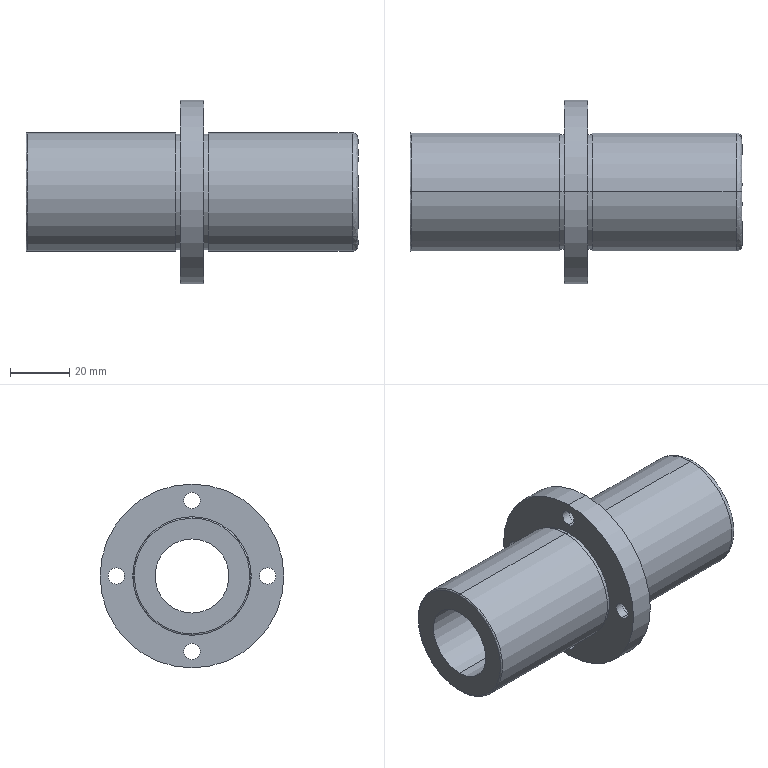Part | SolidWorks | features BaseBody 1 | 1 solid | 42 faces | box 112 x 62 x 62 mm | volume 97978 mm3 | cylinder 28 | plane 10 | spline 4 | commonest cylinder face diameters 5.5 x8 9 x8 39 x4 40 x4 25 x2 62 x2